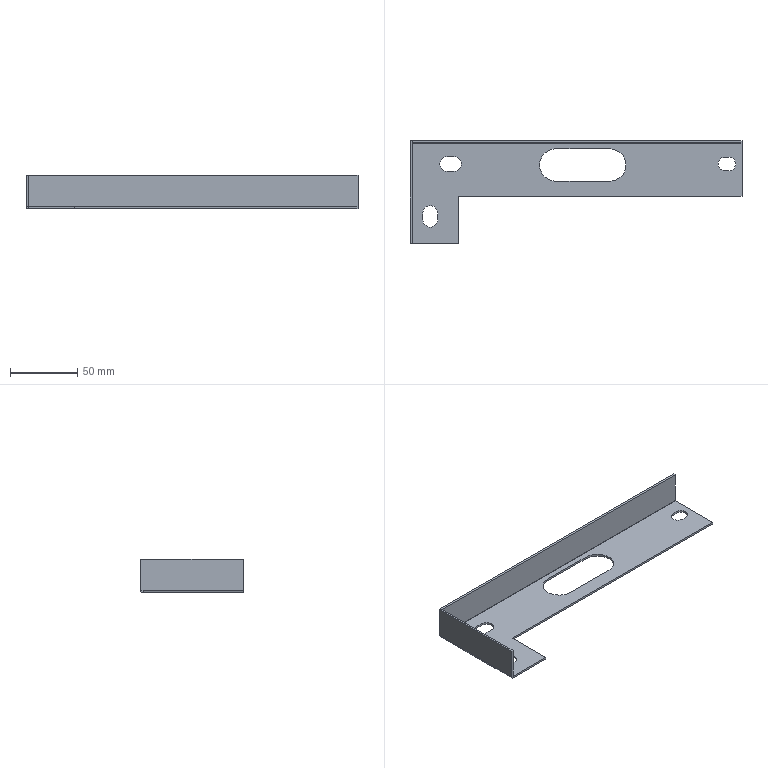Part | SolidWorks | features ICE 5, EdgeFlange 3, Cut 2, FlatPattern 1, SMBaseFlange 1, SheetMetal 1 | 1 solid | 44 faces | box 246 x 76 x 25 mm | volume 25378 mm3 | plane 29 | cylinder 15 | commonest cylinder face diameters 11 x5 10 x3 24 x3 0.4 x2 3.4 x2
STEP:
#1=CARTESIAN_POINT('',(37.,20.,-1.5));
#2=VERTEX_POINT('',#1);
#3=CARTESIAN_POINT('',(25.,32.,-1.5));
#4=VERTEX_POINT('',#3);
#5=CARTESIAN_POINT('',(25.,20.,-1.5));
#6=DIRECTION('',(0.,0.,1.));
#7=DIRECTION('',(1.,0.,0.));
#8=AXIS2_PLACEMENT_3D('',#5,#6,#7);
#9=CIRCLE('',#8,12.);
#10=EDGE_CURVE('',#2,#4,#9,.T.);
#11=ORIENTED_EDGE('',*,*,#10,.F.);
#12=CARTESIAN_POINT('',(37.,20.,0.));
#13=VERTEX_POINT('',#12);
#14=CARTESIAN_POINT('',(37.,20.,-10.));
#15=DIRECTION('',(0.,0.,1.));
#16=VECTOR('',#15,1000.);
#17=LINE('',#14,#16);
#18=EDGE_CURVE('',#2,#13,#17,.T.);
#19=ORIENTED_EDGE('',*,*,#18,.T.);
#20=CARTESIAN_POINT('',(25.,32.,0.));
#21=VERTEX_POINT('',#20);
#22=CARTESIAN_POINT('',(25.,20.,0.));
#23=DIRECTION('',(0.,0.,1.));
#24=DIRECTION('',(1.,0.,0.));
#25=AXIS2_PLACEMENT_3D('',#22,#23,#24);
#26=CIRCLE('',#25,12.);
#27=EDGE_CURVE('',#13,#21,#26,.T.);
#28=ORIENTED_EDGE('',*,*,#27,.T.);
#29=CARTESIAN_POINT('',(25.,32.,-10.));
#30=DIRECTION('',(0.,0.,1.));
#31=VECTOR('',#30,1000.);
#32=LINE('',#29,#31);
#33=EDGE_CURVE('',#4,#21,#32,.T.);
#34=ORIENTED_EDGE('',*,*,#33,.F.);
#35=EDGE_LOOP('',(#11,#19,#28,#34));
#36=FACE_OUTER_BOUND('',#35,.T.);
#37=CARTESIAN_POINT('',(25.,20.,-10.));
#38=DIRECTION('',(0.,0.,1.));
#39=DIRECTION('',(1.,0.,0.));
#40=AXIS2_PLACEMENT_3D('',#37,#38,#39);
#41=CYLINDRICAL_SURFACE('',#40,12.);
#42=ADVANCED_FACE('',(#36),#41,.F.);
#43=CARTESIAN_POINT('',(118.3,20.8,-1.5));
#44=VERTEX_POINT('',#43);
#45=CARTESIAN_POINT('',(113.3,25.8,-1.5));
#46=VERTEX_POINT('',#45);
#47=CARTESIAN_POINT('',(113.3,20.8,-1.5));
#48=DIRECTION('',(0.,0.,1.));
#49=DIRECTION('',(1.,0.,0.));
#50=AXIS2_PLACEMENT_3D('',#47,#48,#49);
#51=CIRCLE('',#50,5.);
#52=EDGE_CURVE('',#44,#46,#51,.T.);
#53=ORIENTED_EDGE('',*,*,#52,.F.);
#54=CARTESIAN_POINT('',(118.3,20.8,0.));
#55=VERTEX_POINT('',#54);
#56=CARTESIAN_POINT('',(118.3,20.8,-10.));
#57=DIRECTION('',(0.,0.,1.));
#58=VECTOR('',#57,1000.);
#59=LINE('',#56,#58);
#60=EDGE_CURVE('',#44,#55,#59,.T.);
#61=ORIENTED_EDGE('',*,*,#60,.T.);
#62=CARTESIAN_POINT('',(113.3,25.8,0.));
#63=VERTEX_POINT('',#62);
#64=CARTESIAN_POINT('',(113.3,20.8,0.));
#65=DIRECTION('',(0.,0.,1.));
#66=DIRECTION('',(1.,0.,0.));
#67=AXIS2_PLACEMENT_3D('',#64,#65,#66);
#68=CIRCLE('',#67,5.);
#69=EDGE_CURVE('',#55,#63,#68,.T.);
#70=ORIENTED_EDGE('',*,*,#69,.T.);
#71=CARTESIAN_POINT('',(113.3,25.8,-10.));
#72=DIRECTION('',(0.,0.,1.));
#73=VECTOR('',#72,1000.);
#74=LINE('',#71,#73);
#75=EDGE_CURVE('',#46,#63,#74,.T.);
#76=ORIENTED_EDGE('',*,*,#75,.F.);
#77=EDGE_LOOP('',(#53,#61,#70,#76));
#78=FACE_OUTER_BOUND('',#77,.T.);
#79=CARTESIAN_POINT('',(113.3,20.8,-10.));
#80=DIRECTION('',(0.,0.,1.));
#81=DIRECTION('',(1.,0.,0.));
#82=AXIS2_PLACEMENT_3D('',#79,#80,#81);
#83=CYLINDRICAL_SURFACE('',#82,5.);
#84=ADVANCED_FACE('',(#78),#83,.F.);
#85=CARTESIAN_POINT('',(-85.,20.8,-1.5));
#86=VERTEX_POINT('',#85);
#87=CARTESIAN_POINT('',(-90.5,26.3,-1.5));
#88=VERTEX_POINT('',#87);
#89=CARTESIAN_POINT('',(-90.5,20.8,-1.5));
#90=DIRECTION('',(0.,0.,1.));
#91=DIRECTION('',(1.,0.,0.));
#92=AXIS2_PLACEMENT_3D('',#89,#90,#91);
#93=CIRCLE('',#92,5.5);
#94=EDGE_CURVE('',#86,#88,#93,.T.);
#95=ORIENTED_EDGE('',*,*,#94,.F.);
#96=CARTESIAN_POINT('',(-85.,20.8,0.));
#97=VERTEX_POINT('',#96);
#98=CARTESIAN_POINT('',(-85.,20.8,-10.));
#99=DIRECTION('',(0.,0.,1.));
#100=VECTOR('',#99,1000.);
#101=LINE('',#98,#100);
#102=EDGE_CURVE('',#86,#97,#101,.T.);
#103=ORIENTED_EDGE('',*,*,#102,.T.);
#104=CARTESIAN_POINT('',(-90.5,26.3,0.));
#105=VERTEX_POINT('',#104);
#106=CARTESIAN_POINT('',(-90.5,20.8,0.));
#107=DIRECTION('',(0.,0.,1.));
#108=DIRECTION('',(1.,0.,0.));
#109=AXIS2_PLACEMENT_3D('',#106,#107,#108);
#110=CIRCLE('',#109,5.5);
#111=EDGE_CURVE('',#97,#105,#110,.T.);
#112=ORIENTED_EDGE('',*,*,#111,.T.);
#113=CARTESIAN_POINT('',(-90.5,26.3,-10.));
#114=DIRECTION('',(0.,0.,1.));
#115=VECTOR('',#114,1000.);
#116=LINE('',#113,#115);
#117=EDGE_CURVE('',#88,#105,#116,.T.);
#118=ORIENTED_EDGE('',*,*,#117,.F.);
#119=EDGE_LOOP('',(#95,#103,#112,#118));
#120=FACE_OUTER_BOUND('',#119,.T.);
#121=CARTESIAN_POINT('',(-90.5,20.8,-10.));
#122=DIRECTION('',(0.,0.,1.));
#123=DIRECTION('',(1.,0.,0.));
#124=AXIS2_PLACEMENT_3D('',#121,#122,#123);
#125=CYLINDRICAL_SURFACE('',#124,5.5);
#126=ADVANCED_FACE('',(#120),#125,.F.);
#127=CARTESIAN_POINT('',(-123.,36.3,0.2));
#128=VERTEX_POINT('',#127);
#129=CARTESIAN_POINT('',(-121.5,36.3,0.2));
#130=VERTEX_POINT('',#129);
#131=CARTESIAN_POINT('',(-123.,36.3,0.2));
#132=DIRECTION('',(1.,0.,0.));
#133=VECTOR('',#132,1000.);
#134=LINE('',#131,#133);
#135=EDGE_CURVE('',#128,#130,#134,.T.);
#136=ORIENTED_EDGE('',*,*,#135,.F.);
#137=CARTESIAN_POINT('',(-123.,38.,0.2));
#138=VERTEX_POINT('',#137);
#139=CARTESIAN_POINT('',(-123.,38.,0.2));
#140=DIRECTION('',(0.,1.,0.));
#141=VECTOR('',#140,1000.);
#142=LINE('',#139,#141);
#143=EDGE_CURVE('',#128,#138,#142,.T.);
#144=ORIENTED_EDGE('',*,*,#143,.T.);
#145=CARTESIAN_POINT('',(-121.5,38.,0.2));
#146=VERTEX_POINT('',#145);
#147=CARTESIAN_POINT('',(-123.,38.,0.2));
#148=DIRECTION('',(-1.,0.,0.));
#149=VECTOR('',#148,1000.);
#150=LINE('',#147,#149);
#151=EDGE_CURVE('',#146,#138,#150,.T.);
#152=ORIENTED_EDGE('',*,*,#151,.F.);
#153=CARTESIAN_POINT('',(-121.5,38.,0.2));
#154=DIRECTION('',(0.,-1.,0.));
#155=VECTOR('',#154,1000.);
#156=LINE('',#153,#155);
#157=EDGE_CURVE('',#146,#130,#156,.T.);
#158=ORIENTED_EDGE('',*,*,#157,.T.);
#159=EDGE_LOOP('',(#136,#144,#152,#158));
#160=FACE_OUTER_BOUND('',#159,.T.);
#161=CARTESIAN_POINT('',(0.,0.,0.2));
#162=DIRECTION('',(0.,0.,-1.));
#163=DIRECTION('',(-1.,0.,0.));
#164=AXIS2_PLACEMENT_3D('',#161,#162,#163);
#165=PLANE('',#164);
#166=ADVANCED_FACE('',(#160),#165,.T.);
#167=CARTESIAN_POINT('',(-123.,-38.,0.2));
#168=VERTEX_POINT('',#167);
#169=CARTESIAN_POINT('',(-123.,38.,0.2));
#170=DIRECTION('',(0.,1.,0.));
#171=VECTOR('',#170,1000.);
#172=LINE('',#169,#171);
#173=EDGE_CURVE('',#168,#128,#172,.T.);
#174=ORIENTED_EDGE('',*,*,#173,.T.);
#175=CARTESIAN_POINT('',(-121.3,36.3,-1.5));
#176=VERTEX_POINT('',#175);
#177=CARTESIAN_POINT('',(-121.3,36.3,0.2));
#178=DIRECTION('',(0.,-1.,0.));
#179=DIRECTION('',(0.,0.,1.));
#180=AXIS2_PLACEMENT_3D('',#177,#178,#179);
#181=CIRCLE('',#180,1.7);
#182=EDGE_CURVE('',#128,#176,#181,.T.);
#183=ORIENTED_EDGE('',*,*,#182,.T.);
#184=CARTESIAN_POINT('',(-121.3,-38.,-1.5));
#185=VERTEX_POINT('',#184);
#186=CARTESIAN_POINT('',(-121.3,-38.,-1.5));
#187=DIRECTION('',(0.,1.,0.));
#188=VECTOR('',#187,1000.);
#189=LINE('',#186,#188);
#190=EDGE_CURVE('',#185,#176,#189,.T.);
#191=ORIENTED_EDGE('',*,*,#190,.F.);
#192=CARTESIAN_POINT('',(-121.3,-38.,0.2));
#193=DIRECTION('',(0.,-1.,0.));
#194=DIRECTION('',(0.,0.,-1.));
#195=AXIS2_PLACEMENT_3D('',#192,#193,#194);
#196=CIRCLE('',#195,1.7);
#197=EDGE_CURVE('',#168,#185,#196,.T.);
#198=ORIENTED_EDGE('',*,*,#197,.F.);
#199=EDGE_LOOP('',(#174,#183,#191,#198));
#200=FACE_OUTER_BOUND('',#199,.T.);
#201=CARTESIAN_POINT('',(-121.3,-38.,0.2));
#202=DIRECTION('',(0.,-1.,0.));
#203=DIRECTION('',(-1.,0.,0.));
#204=AXIS2_PLACEMENT_3D('',#201,#202,#203);
#205=CYLINDRICAL_SURFACE('',#204,1.7);
#206=ADVANCED_FACE('',(#200),#205,.T.);
#207=CARTESIAN_POINT('',(-15.,32.,-1.5));
#208=VERTEX_POINT('',#207);
#209=CARTESIAN_POINT('',(0.,32.,-1.5));
#210=DIRECTION('',(-1.,0.,0.));
#211=VECTOR('',#210,1000.);
#212=LINE('',#209,#211);
#213=EDGE_CURVE('',#4,#208,#212,.T.);
#214=ORIENTED_EDGE('',*,*,#213,.T.);
#215=CARTESIAN_POINT('',(-15.,8.,-1.5));
#216=VERTEX_POINT('',#215);
#217=CARTESIAN_POINT('',(-15.,20.,-1.5));
#218=DIRECTION('',(0.,0.,1.));
#219=DIRECTION('',(1.,0.,0.));
#220=AXIS2_PLACEMENT_3D('',#217,#218,#219);
#221=CIRCLE('',#220,12.);
#222=EDGE_CURVE('',#208,#216,#221,.T.);
#223=ORIENTED_EDGE('',*,*,#222,.T.);
#224=CARTESIAN_POINT('',(25.,8.,-1.5));
#225=VERTEX_POINT('',#224);
#226=CARTESIAN_POINT('',(0.,8.,-1.5));
#227=DIRECTION('',(1.,0.,0.));
#228=VECTOR('',#227,1000.);
#229=LINE('',#226,#228);
#230=EDGE_CURVE('',#216,#225,#229,.T.);
#231=ORIENTED_EDGE('',*,*,#230,.T.);
#232=CARTESIAN_POINT('',(25.,20.,-1.5));
#233=DIRECTION('',(0.,0.,1.));
#234=DIRECTION('',(1.,0.,0.));
#235=AXIS2_PLACEMENT_3D('',#232,#233,#234);
#236=CIRCLE('',#235,12.);
#237=EDGE_CURVE('',#225,#2,#236,.T.);
#238=ORIENTED_EDGE('',*,*,#237,.T.);
#239=ORIENTED_EDGE('',*,*,#10,.T.);
#240=EDGE_LOOP('',(#214,#223,#231,#238,#239));
#241=FACE_BOUND('',#240,.T.);
#242=CARTESIAN_POINT('',(110.3,25.8,-1.5));
#243=VERTEX_POINT('',#242);
#244=CARTESIAN_POINT('',(0.,25.8,-1.5));
#245=DIRECTION('',(-1.,0.,0.));
#246=VECTOR('',#245,1000.);
#247=LINE('',#244,#246);
#248=EDGE_CURVE('',#46,#243,#247,.T.);
#249=ORIENTED_EDGE('',*,*,#248,.T.);
#250=CARTESIAN_POINT('',(110.3,15.8,-1.5));
#251=VERTEX_POINT('',#250);
#252=CARTESIAN_POINT('',(110.3,20.8,-1.5));
#253=DIRECTION('',(0.,0.,1.));
#254=DIRECTION('',(1.,0.,0.));
#255=AXIS2_PLACEMENT_3D('',#252,#253,#254);
#256=CIRCLE('',#255,5.);
#257=EDGE_CURVE('',#243,#251,#256,.T.);
#258=ORIENTED_EDGE('',*,*,#257,.T.);
#259=CARTESIAN_POINT('',(113.3,15.8,-1.5));
#260=VERTEX_POINT('',#259);
#261=CARTESIAN_POINT('',(0.,15.8,-1.5));
#262=DIRECTION('',(1.,0.,0.));
#263=VECTOR('',#262,1000.);
#264=LINE('',#261,#263);
#265=EDGE_CURVE('',#251,#260,#264,.T.);
#266=ORIENTED_EDGE('',*,*,#265,.T.);
#267=CARTESIAN_POINT('',(113.3,20.8,-1.5));
#268=DIRECTION('',(0.,0.,1.));
#269=DIRECTION('',(1.,0.,0.));
#270=AXIS2_PLACEMENT_3D('',#267,#268,#269);
#271=CIRCLE('',#270,5.);
#272=EDGE_CURVE('',#260,#44,#271,.T.);
#273=ORIENTED_EDGE('',*,*,#272,.T.);
#274=ORIENTED_EDGE('',*,*,#52,.T.);
#275=EDGE_LOOP('',(#249,#258,#266,#273,#274));
#276=FACE_BOUND('',#275,.T.);
#277=CARTESIAN_POINT('',(-95.5,26.3,-1.5));
#278=VERTEX_POINT('',#277);
#279=CARTESIAN_POINT('',(0.,26.3,-1.5));
#280=DIRECTION('',(-1.,0.,0.));
#281=VECTOR('',#280,1000.);
#282=LINE('',#279,#281);
#283=EDGE_CURVE('',#88,#278,#282,.T.);
#284=ORIENTED_EDGE('',*,*,#283,.T.);
#285=CARTESIAN_POINT('',(-95.5,15.3,-1.5));
#286=VERTEX_POINT('',#285);
#287=CARTESIAN_POINT('',(-95.5,20.8,-1.5));
#288=DIRECTION('',(0.,0.,1.));
#289=DIRECTION('',(1.,0.,0.));
#290=AXIS2_PLACEMENT_3D('',#287,#288,#289);
#291=CIRCLE('',#290,5.5);
#292=EDGE_CURVE('',#278,#286,#291,.T.);
#293=ORIENTED_EDGE('',*,*,#292,.T.);
#294=CARTESIAN_POINT('',(-90.5,15.3,-1.5));
#295=VERTEX_POINT('',#294);
#296=CARTESIAN_POINT('',(0.,15.3,-1.5));
#297=DIRECTION('',(1.,0.,0.));
#298=VECTOR('',#297,1000.);
#299=LINE('',#296,#298);
#300=EDGE_CURVE('',#286,#295,#299,.T.);
#301=ORIENTED_EDGE('',*,*,#300,.T.);
#302=CARTESIAN_POINT('',(-90.5,20.8,-1.5));
#303=DIRECTION('',(0.,0.,1.));
#304=DIRECTION('',(1.,0.,0.));
#305=AXIS2_PLACEMENT_3D('',#302,#303,#304);
#306=CIRCLE('',#305,5.5);
#307=EDGE_CURVE('',#295,#86,#306,.T.);
#308=ORIENTED_EDGE('',*,*,#307,.T.);
#309=ORIENTED_EDGE('',*,*,#94,.T.);
#310=EDGE_LOOP('',(#284,#293,#301,#308,#309));
#311=FACE_BOUND('',#310,.T.);
#312=CARTESIAN_POINT('',(-102.5,-20.5,-1.5));
#313=VERTEX_POINT('',#312);
#314=CARTESIAN_POINT('',(-102.5,-15.5,-1.5));
#315=VERTEX_POINT('',#314);
#316=CARTESIAN_POINT('',(-102.5,0.,-1.5));
#317=DIRECTION('',(0.,1.,0.));
#318=VECTOR('',#317,1000.);
#319=LINE('',#316,#318);
#320=EDGE_CURVE('',#313,#315,#319,.T.);
#321=ORIENTED_EDGE('',*,*,#320,.T.);
#322=CARTESIAN_POINT('',(-113.5,-15.5,-1.5));
#323=VERTEX_POINT('',#322);
#324=CARTESIAN_POINT('',(-108.,-15.5,-1.5));
#325=DIRECTION('',(0.,0.,1.));
#326=DIRECTION('',(1.,0.,0.));
#327=AXIS2_PLACEMENT_3D('',#324,#325,#326);
#328=CIRCLE('',#327,5.5);
#329=EDGE_CURVE('',#315,#323,#328,.T.);
#330=ORIENTED_EDGE('',*,*,#329,.T.);
#331=CARTESIAN_POINT('',(-113.5,-20.5,-1.5));
#332=VERTEX_POINT('',#331);
#333=CARTESIAN_POINT('',(-113.5,0.,-1.5));
#334=DIRECTION('',(0.,-1.,0.));
#335=VECTOR('',#334,1000.);
#336=LINE('',#333,#335);
#337=EDGE_CURVE('',#323,#332,#336,.T.);
#338=ORIENTED_EDGE('',*,*,#337,.T.);
#339=CARTESIAN_POINT('',(-108.,-20.5,-1.5));
#340=DIRECTION('',(0.,0.,1.));
#341=DIRECTION('',(1.,0.,0.));
#342=AXIS2_PLACEMENT_3D('',#339,#340,#341);
#343=CIRCLE('',#342,5.5);
#344=EDGE_CURVE('',#332,#313,#343,.T.);
#345=ORIENTED_EDGE('',*,*,#344,.T.);
#346=EDGE_LOOP('',(#321,#330,#338,#345));
#347=FACE_BOUND('',#346,.T.);
#348=CARTESIAN_POINT('',(123.,-3.,-1.5));
#349=VERTEX_POINT('',#348);
#350=CARTESIAN_POINT('',(123.,36.3,-1.5));
#351=VERTEX_POINT('',#350);
#352=CARTESIAN_POINT('',(123.,38.,-1.5));
#353=DIRECTION('',(0.,1.,0.));
#354=VECTOR('',#353,1000.);
#355=LINE('',#352,#354);
#356=EDGE_CURVE('',#349,#351,#355,.T.);
#357=ORIENTED_EDGE('',*,*,#356,.F.);
#358=CARTESIAN_POINT('',(-87.,-3.,-1.5));
#359=VERTEX_POINT('',#358);
#360=CARTESIAN_POINT('',(123.,-3.,-1.5));
#361=DIRECTION('',(1.,0.,0.));
#362=VECTOR('',#361,1000.);
#363=LINE('',#360,#362);
#364=EDGE_CURVE('',#359,#349,#363,.T.);
#365=ORIENTED_EDGE('',*,*,#364,.F.);
#366=CARTESIAN_POINT('',(-87.,-38.,-1.5));
#367=VERTEX_POINT('',#366);
#368=CARTESIAN_POINT('',(-87.,-38.,-1.5));
#369=DIRECTION('',(0.,1.,0.));
#370=VECTOR('',#369,1000.);
#371=LINE('',#368,#370);
#372=EDGE_CURVE('',#367,#359,#371,.T.);
#373=ORIENTED_EDGE('',*,*,#372,.F.);
#374=CARTESIAN_POINT('',(-123.,-38.,-1.5));
#375=DIRECTION('',(1.,0.,0.));
#376=VECTOR('',#375,1000.);
#377=LINE('',#374,#376);
#378=EDGE_CURVE('',#185,#367,#377,.T.);
#379=ORIENTED_EDGE('',*,*,#378,.F.);
#380=ORIENTED_EDGE('',*,*,#190,.T.);
#381=CARTESIAN_POINT('',(-121.3,36.3,-1.5));
#382=DIRECTION('',(1.,0.,0.));
#383=VECTOR('',#382,1000.);
#384=LINE('',#381,#383);
#385=EDGE_CURVE('',#176,#351,#384,.T.);
#386=ORIENTED_EDGE('',*,*,#385,.T.);
#387=EDGE_LOOP('',(#357,#365,#373,#379,#380,#386));
#388=FACE_OUTER_BOUND('',#387,.T.);
#389=CARTESIAN_POINT('',(0.,0.,-1.5));
#390=DIRECTION('',(0.,0.,1.));
#391=DIRECTION('',(1.,0.,0.));
#392=AXIS2_PLACEMENT_3D('',#389,#390,#391);
#393=PLANE('',#392);
#394=ADVANCED_FACE('',(#241,#276,#311,#347,#388),#393,.F.);
#395=CARTESIAN_POINT('',(123.,-3.,0.));
#396=VERTEX_POINT('',#395);
#397=CARTESIAN_POINT('',(-87.,-3.,0.));
#398=VERTEX_POINT('',#397);
#399=CARTESIAN_POINT('',(0.,-3.,0.));
#400=DIRECTION('',(-1.,0.,0.));
#401=VECTOR('',#400,1000.);
#402=LINE('',#399,#401);
#403=EDGE_CURVE('',#396,#398,#402,.T.);
#404=ORIENTED_EDGE('',*,*,#403,.F.);
#405=CARTESIAN_POINT('',(123.,36.3,0.));
#406=VERTEX_POINT('',#405);
#407=CARTESIAN_POINT('',(123.,38.,0.));
#408=DIRECTION('',(0.,1.,0.));
#409=VECTOR('',#408,1000.);
#410=LINE('',#407,#409);
#411=EDGE_CURVE('',#396,#406,#410,.T.);
#412=ORIENTED_EDGE('',*,*,#411,.T.);
#413=CARTESIAN_POINT('',(-121.3,36.3,0.));
#414=VERTEX_POINT('',#413);
#415=CARTESIAN_POINT('',(-121.3,36.3,0.));
#416=DIRECTION('',(1.,0.,0.));
#417=VECTOR('',#416,1000.);
#418=LINE('',#415,#417);
#419=EDGE_CURVE('',#414,#406,#418,.T.);
#420=ORIENTED_EDGE('',*,*,#419,.F.);
#421=CARTESIAN_POINT('',(-121.3,-38.,0.));
#422=VERTEX_POINT('',#421);
#423=CARTESIAN_POINT('',(-121.3,-38.,0.));
#424=DIRECTION('',(0.,1.,0.));
#425=VECTOR('',#424,1000.);
#426=LINE('',#423,#425);
#427=EDGE_CURVE('',#422,#414,#426,.T.);
#428=ORIENTED_EDGE('',*,*,#427,.F.);
#429=CARTESIAN_POINT('',(-87.,-38.,0.));
#430=VERTEX_POINT('',#429);
#431=CARTESIAN_POINT('',(-123.,-38.,0.));
#432=DIRECTION('',(1.,0.,0.));
#433=VECTOR('',#432,1000.);
#434=LINE('',#431,#433);
#435=EDGE_CURVE('',#422,#430,#434,.T.);
#436=ORIENTED_EDGE('',*,*,#435,.T.);
#437=CARTESIAN_POINT('',(-87.,0.,0.));
#438=DIRECTION('',(0.,-1.,0.));
#439=VECTOR('',#438,1000.);
#440=LINE('',#437,#439);
#441=EDGE_CURVE('',#398,#430,#440,.T.);
#442=ORIENTED_EDGE('',*,*,#441,.F.);
#443=EDGE_LOOP('',(#404,#412,#420,#428,#436,#442));
#444=FACE_OUTER_BOUND('',#443,.T.);
#445=CARTESIAN_POINT('',(-15.,32.,0.));
#446=VERTEX_POINT('',#445);
#447=CARTESIAN_POINT('',(-15.,8.,0.));
#448=VERTEX_POINT('',#447);
#449=CARTESIAN_POINT('',(-15.,20.,0.));
#450=DIRECTION('',(0.,0.,1.));
#451=DIRECTION('',(1.,0.,0.));
#452=AXIS2_PLACEMENT_3D('',#449,#450,#451);
#453=CIRCLE('',#452,12.);
#454=EDGE_CURVE('',#446,#448,#453,.T.);
#455=ORIENTED_EDGE('',*,*,#454,.F.);
#456=CARTESIAN_POINT('',(-15.,32.,0.));
#457=DIRECTION('',(-1.,0.,0.));
#458=VECTOR('',#457,1000.);
#459=LINE('',#456,#458);
#460=EDGE_CURVE('',#21,#446,#459,.T.);
#461=ORIENTED_EDGE('',*,*,#460,.F.);
#462=ORIENTED_EDGE('',*,*,#27,.F.);
#463=CARTESIAN_POINT('',(25.,8.,0.));
#464=VERTEX_POINT('',#463);
#465=CARTESIAN_POINT('',(25.,20.,0.));
#466=DIRECTION('',(0.,0.,1.));
#467=DIRECTION('',(1.,0.,0.));
#468=AXIS2_PLACEMENT_3D('',#465,#466,#467);
#469=CIRCLE('',#468,12.);
#470=EDGE_CURVE('',#464,#13,#469,.T.);
#471=ORIENTED_EDGE('',*,*,#470,.F.);
#472=CARTESIAN_POINT('',(-15.,8.,0.));
#473=DIRECTION('',(1.,0.,0.));
#474=VECTOR('',#473,1000.);
#475=LINE('',#472,#474);
#476=EDGE_CURVE('',#448,#464,#475,.T.);
#477=ORIENTED_EDGE('',*,*,#476,.F.);
#478=EDGE_LOOP('',(#455,#461,#462,#471,#477));
#479=FACE_BOUND('',#478,.T.);
#480=CARTESIAN_POINT('',(110.3,25.8,0.));
#481=VERTEX_POINT('',#480);
#482=CARTESIAN_POINT('',(110.3,15.8,0.));
#483=VERTEX_POINT('',#482);
#484=CARTESIAN_POINT('',(110.3,20.8,0.));
#485=DIRECTION('',(0.,0.,1.));
#486=DIRECTION('',(1.,0.,0.));
#487=AXIS2_PLACEMENT_3D('',#484,#485,#486);
#488=CIRCLE('',#487,5.);
#489=EDGE_CURVE('',#481,#483,#488,.T.);
#490=ORIENTED_EDGE('',*,*,#489,.F.);
#491=CARTESIAN_POINT('',(110.3,25.8,0.));
#492=DIRECTION('',(-1.,0.,0.));
#493=VECTOR('',#492,1000.);
#494=LINE('',#491,#493);
#495=EDGE_CURVE('',#63,#481,#494,.T.);
#496=ORIENTED_EDGE('',*,*,#495,.F.);
#497=ORIENTED_EDGE('',*,*,#69,.F.);
#498=CARTESIAN_POINT('',(113.3,15.8,0.));
#499=VERTEX_POINT('',#498);
#500=CARTESIAN_POINT('',(113.3,20.8,0.));
#501=DIRECTION('',(0.,0.,1.));
#502=DIRECTION('',(1.,0.,0.));
#503=AXIS2_PLACEMENT_3D('',#500,#501,#502);
#504=CIRCLE('',#503,5.);
#505=EDGE_CURVE('',#499,#55,#504,.T.);
#506=ORIENTED_EDGE('',*,*,#505,.F.);
#507=CARTESIAN_POINT('',(110.3,15.8,0.));
#508=DIRECTION('',(1.,0.,0.));
#509=VECTOR('',#508,1000.);
#510=LINE('',#507,#509);
#511=EDGE_CURVE('',#483,#499,#510,.T.);
#512=ORIENTED_EDGE('',*,*,#511,.F.);
#513=EDGE_LOOP('',(#490,#496,#497,#506,#512));
#514=FACE_BOUND('',#513,.T.);
#515=CARTESIAN_POINT('',(-95.5,26.3,0.));
#516=VERTEX_POINT('',#515);
#517=CARTESIAN_POINT('',(-95.5,15.3,0.));
#518=VERTEX_POINT('',#517);
#519=CARTESIAN_POINT('',(-95.5,20.8,0.));
#520=DIRECTION('',(0.,0.,1.));
#521=DIRECTION('',(1.,0.,0.));
#522=AXIS2_PLACEMENT_3D('',#519,#520,#521);
#523=CIRCLE('',#522,5.5);
#524=EDGE_CURVE('',#516,#518,#523,.T.);
#525=ORIENTED_EDGE('',*,*,#524,.F.);
#526=CARTESIAN_POINT('',(-95.5,26.3,0.));
#527=DIRECTION('',(-1.,0.,0.));
#528=VECTOR('',#527,1000.);
#529=LINE('',#526,#528);
#530=EDGE_CURVE('',#105,#516,#529,.T.);
#531=ORIENTED_EDGE('',*,*,#530,.F.);
#532=ORIENTED_EDGE('',*,*,#111,.F.);
#533=CARTESIAN_POINT('',(-90.5,15.3,0.));
#534=VERTEX_POINT('',#533);
#535=CARTESIAN_POINT('',(-90.5,20.8,0.));
#536=DIRECTION('',(0.,0.,1.));
#537=DIRECTION('',(1.,0.,0.));
#538=AXIS2_PLACEMENT_3D('',#535,#536,#537);
#539=CIRCLE('',#538,5.5);
#540=EDGE_CURVE('',#534,#97,#539,.T.);
#541=ORIENTED_EDGE('',*,*,#540,.F.);
#542=CARTESIAN_POINT('',(-95.5,15.3,0.));
#543=DIRECTION('',(1.,0.,0.));
#544=VECTOR('',#543,1000.);
#545=LINE('',#542,#544);
#546=EDGE_CURVE('',#518,#534,#545,.T.);
#547=ORIENTED_EDGE('',*,*,#546,.F.);
#548=EDGE_LOOP('',(#525,#531,#532,#541,#547));
#549=FACE_BOUND('',#548,.T.);
#550=CARTESIAN_POINT('',(-102.5,-15.5,0.));
#551=VERTEX_POINT('',#550);
#552=CARTESIAN_POINT('',(-113.5,-15.5,0.));
#553=VERTEX_POINT('',#552);
#554=CARTESIAN_POINT('',(-108.,-15.5,0.));
#555=DIRECTION('',(0.,0.,1.));
#556=DIRECTION('',(1.,0.,0.));
#557=AXIS2_PLACEMENT_3D('',#554,#555,#556);
#558=CIRCLE('',#557,5.5);
#559=EDGE_CURVE('',#551,#553,#558,.T.);
#560=ORIENTED_EDGE('',*,*,#559,.F.);
#561=CARTESIAN_POINT('',(-102.5,-20.5,0.));
#562=VERTEX_POINT('',#561);
#563=CARTESIAN_POINT('',(-102.5,-15.5,0.));
#564=DIRECTION('',(0.,1.,0.));
#565=VECTOR('',#564,1000.);
#566=LINE('',#563,#565);
#567=EDGE_CURVE('',#562,#551,#566,.T.);
#568=ORIENTED_EDGE('',*,*,#567,.F.);
#569=CARTESIAN_POINT('',(-113.5,-20.5,0.));
#570=VERTEX_POINT('',#569);
#571=CARTESIAN_POINT('',(-108.,-20.5,0.));
#572=DIRECTION('',(0.,0.,1.));
#573=DIRECTION('',(1.,0.,0.));
#574=AXIS2_PLACEMENT_3D('',#571,#572,#573);
#575=CIRCLE('',#574,5.5);
#576=EDGE_CURVE('',#570,#562,#575,.T.);
#577=ORIENTED_EDGE('',*,*,#576,.F.);
#578=CARTESIAN_POINT('',(-113.5,-15.5,0.));
#579=DIRECTION('',(0.,-1.,0.));
#580=VECTOR('',#579,1000.);
#581=LINE('',#578,#580);
#582=EDGE_CURVE('',#553,#570,#581,.T.);
#583=ORIENTED_EDGE('',*,*,#582,.F.);
#584=EDGE_LOOP('',(#560,#568,#577,#583));
#585=FACE_BOUND('',#584,.T.);
#586=CARTESIAN_POINT('',(0.,0.,0.));
#587=DIRECTION('',(0.,0.,1.));
#588=DIRECTION('',(1.,0.,0.));
#589=AXIS2_PLACEMENT_3D('',#586,#587,#588);
#590=PLANE('',#589);
#591=ADVANCED_FACE('',(#444,#479,#514,#549,#585),#590,.T.);
#592=CARTESIAN_POINT('',(-87.,-38.,8.5));
#593=DIRECTION('',(0.,0.,-1.));
#594=VECTOR('',#593,1000.);
#595=LINE('',#592,#594);
#596=EDGE_CURVE('',#430,#367,#595,.T.);
#597=ORIENTED_EDGE('',*,*,#596,.F.);
#598=ORIENTED_EDGE('',*,*,#435,.F.);
#599=CARTESIAN_POINT('',(-121.3,-38.,0.));
#600=DIRECTION('',(0.,0.,-1.));
#601=VECTOR('',#600,1000.);
#602=LINE('',#599,#601);
#603=EDGE_CURVE('',#422,#185,#602,.T.);
#604=ORIENTED_EDGE('',*,*,#603,.T.);
#605=ORIENTED_EDGE('',*,*,#378,.T.);
#606=EDGE_LOOP('',(#597,#598,#604,#605));
#607=FACE_OUTER_BOUND('',#606,.T.);
#608=CARTESIAN_POINT('',(-123.,-38.,-1.5));
#609=DIRECTION('',(0.,-1.,0.));
#610=DIRECTION('',(0.,0.,-1.));
#611=AXIS2_PLACEMENT_3D('',#608,#609,#610);
#612=PLANE('',#611);
#613=ADVANCED_FACE('',(#607),#612,.T.);
#614=CARTESIAN_POINT('',(123.,-3.,-1.5));
#615=DIRECTION('',(0.,0.,1.));
#616=VECTOR('',#615,1000.);
#617=LINE('',#614,#616);
#618=EDGE_CURVE('',#349,#396,#617,.T.);
#619=ORIENTED_EDGE('',*,*,#618,.F.);
#620=ORIENTED_EDGE('',*,*,#356,.T.);
#621=CARTESIAN_POINT('',(123.,36.3,0.));
#622=DIRECTION('',(0.,0.,-1.));
#623=VECTOR('',#622,1000.);
#624=LINE('',#621,#623);
#625=EDGE_CURVE('',#406,#351,#624,.T.);
#626=ORIENTED_EDGE('',*,*,#625,.F.);
#627=ORIENTED_EDGE('',*,*,#411,.F.);
#628=EDGE_LOOP('',(#619,#620,#626,#627));
#629=FACE_OUTER_BOUND('',#628,.T.);
#630=CARTESIAN_POINT('',(123.,38.,-1.5));
#631=DIRECTION('',(1.,0.,0.));
#632=DIRECTION('',(0.,0.,-1.));
#633=AXIS2_PLACEMENT_3D('',#630,#631,#632);
#634=PLANE('',#633);
#635=ADVANCED_FACE('',(#629),#634,.T.);
#636=CARTESIAN_POINT('',(-102.5,-15.5,-10.));
#637=DIRECTION('',(0.,0.,1.));
#638=VECTOR('',#637,1000.);
#639=LINE('',#636,#638);
#640=EDGE_CURVE('',#315,#551,#639,.T.);
#641=ORIENTED_EDGE('',*,*,#640,.T.);
#642=ORIENTED_EDGE('',*,*,#559,.T.);
#643=CARTESIAN_POINT('',(-113.5,-15.5,-10.));
#644=DIRECTION('',(0.,0.,1.));
#645=VECTOR('',#644,1000.);
#646=LINE('',#643,#645);
#647=EDGE_CURVE('',#323,#553,#646,.T.);
#648=ORIENTED_EDGE('',*,*,#647,.F.);
#649=ORIENTED_EDGE('',*,*,#329,.F.);
#650=EDGE_LOOP('',(#641,#642,#648,#649));
#651=FACE_OUTER_BOUND('',#650,.T.);
#652=CARTESIAN_POINT('',(-108.,-15.5,-10.));
#653=DIRECTION('',(0.,0.,1.));
#654=DIRECTION('',(1.,0.,0.));
#655=AXIS2_PLACEMENT_3D('',#652,#653,#654);
#656=CYLINDRICAL_SURFACE('',#655,5.5);
#657=ADVANCED_FACE('',(#651),#656,.F.);
#658=CARTESIAN_POINT('',(-102.5,-20.5,-10.));
#659=DIRECTION('',(0.,0.,1.));
#660=VECTOR('',#659,1000.);
#661=LINE('',#658,#660);
#662=EDGE_CURVE('',#313,#562,#661,.T.);
#663=ORIENTED_EDGE('',*,*,#662,.T.);
#664=ORIENTED_EDGE('',*,*,#567,.T.);
#665=ORIENTED_EDGE('',*,*,#640,.F.);
#666=ORIENTED_EDGE('',*,*,#320,.F.);
#667=EDGE_LOOP('',(#663,#664,#665,#666));
#668=FACE_OUTER_BOUND('',#667,.T.);
#669=CARTESIAN_POINT('',(-102.5,-15.5,-10.));
#670=DIRECTION('',(1.,0.,0.));
#671=DIRECTION('',(0.,0.,-1.));
#672=AXIS2_PLACEMENT_3D('',#669,#670,#671);
#673=PLANE('',#672);
#674=ADVANCED_FACE('',(#668),#673,.F.);
#675=CARTESIAN_POINT('',(-113.5,-20.5,-10.));
#676=DIRECTION('',(0.,0.,1.));
#677=VECTOR('',#676,1000.);
#678=LINE('',#675,#677);
#679=EDGE_CURVE('',#332,#570,#678,.T.);
#680=ORIENTED_EDGE('',*,*,#679,.T.);
#681=ORIENTED_EDGE('',*,*,#576,.T.);
#682=ORIENTED_EDGE('',*,*,#662,.F.);
#683=ORIENTED_EDGE('',*,*,#344,.F.);
#684=EDGE_LOOP('',(#680,#681,#682,#683));
#685=FACE_OUTER_BOUND('',#684,.T.);
#686=CARTESIAN_POINT('',(-108.,-20.5,-10.));
#687=DIRECTION('',(0.,0.,1.));
#688=DIRECTION('',(1.,0.,0.));
#689=AXIS2_PLACEMENT_3D('',#686,#687,#688);
#690=CYLINDRICAL_SURFACE('',#689,5.5);
#691=ADVANCED_FACE('',(#685),#690,.F.);
#692=ORIENTED_EDGE('',*,*,#647,.T.);
#693=ORIENTED_EDGE('',*,*,#582,.T.);
#694=ORIENTED_EDGE('',*,*,#679,.F.);
#695=ORIENTED_EDGE('',*,*,#337,.F.);
#696=EDGE_LOOP('',(#692,#693,#694,#695));
#697=FACE_OUTER_BOUND('',#696,.T.);
#698=CARTESIAN_POINT('',(-113.5,-15.5,-10.));
#699=DIRECTION('',(-1.,0.,0.));
#700=DIRECTION('',(0.,0.,1.));
#701=AXIS2_PLACEMENT_3D('',#698,#699,#700);
#702=PLANE('',#701);
#703=ADVANCED_FACE('',(#697),#702,.F.);
#704=CARTESIAN_POINT('',(-95.5,26.3,-10.));
#705=DIRECTION('',(0.,0.,1.));
#706=VECTOR('',#705,1000.);
#707=LINE('',#704,#706);
#708=EDGE_CURVE('',#278,#516,#707,.T.);
#709=ORIENTED_EDGE('',*,*,#708,.T.);
#710=ORIENTED_EDGE('',*,*,#524,.T.);
#711=CARTESIAN_POINT('',(-95.5,15.3,-10.));
#712=DIRECTION('',(0.,0.,1.));
#713=VECTOR('',#712,1000.);
#714=LINE('',#711,#713);
#715=EDGE_CURVE('',#286,#518,#714,.T.);
#716=ORIENTED_EDGE('',*,*,#715,.F.);
#717=ORIENTED_EDGE('',*,*,#292,.F.);
#718=EDGE_LOOP('',(#709,#710,#716,#717));
#719=FACE_OUTER_BOUND('',#718,.T.);
#720=CARTESIAN_POINT('',(-95.5,20.8,-10.));
#721=DIRECTION('',(0.,0.,1.));
#722=DIRECTION('',(1.,0.,0.));
#723=AXIS2_PLACEMENT_3D('',#720,#721,#722);
#724=CYLINDRICAL_SURFACE('',#723,5.5);
#725=ADVANCED_FACE('',(#719),#724,.F.);
#726=ORIENTED_EDGE('',*,*,#117,.T.);
#727=ORIENTED_EDGE('',*,*,#530,.T.);
#728=ORIENTED_EDGE('',*,*,#708,.F.);
#729=ORIENTED_EDGE('',*,*,#283,.F.);
#730=EDGE_LOOP('',(#726,#727,#728,#729));
#731=FACE_OUTER_BOUND('',#730,.T.);
#732=CARTESIAN_POINT('',(-95.5,26.3,-10.));
#733=DIRECTION('',(0.,1.,0.));
#734=DIRECTION('',(0.,0.,1.));
#735=AXIS2_PLACEMENT_3D('',#732,#733,#734);
#736=PLANE('',#735);
#737=ADVANCED_FACE('',(#731),#736,.F.);
#738=ORIENTED_EDGE('',*,*,#102,.F.);
#739=ORIENTED_EDGE('',*,*,#307,.F.);
#740=CARTESIAN_POINT('',(-90.5,15.3,-10.));
#741=DIRECTION('',(0.,0.,1.));
#742=VECTOR('',#741,1000.);
#743=LINE('',#740,#742);
#744=EDGE_CURVE('',#295,#534,#743,.T.);
#745=ORIENTED_EDGE('',*,*,#744,.T.);
#746=ORIENTED_EDGE('',*,*,#540,.T.);
#747=EDGE_LOOP('',(#738,#739,#745,#746));
#748=FACE_OUTER_BOUND('',#747,.T.);
#749=CARTESIAN_POINT('',(-90.5,20.8,-10.));
#750=DIRECTION('',(0.,0.,1.));
#751=DIRECTION('',(1.,0.,0.));
#752=AXIS2_PLACEMENT_3D('',#749,#750,#751);
#753=CYLINDRICAL_SURFACE('',#752,5.5);
#754=ADVANCED_FACE('',(#748),#753,.F.);
#755=ORIENTED_EDGE('',*,*,#715,.T.);
#756=ORIENTED_EDGE('',*,*,#546,.T.);
#757=ORIENTED_EDGE('',*,*,#744,.F.);
#758=ORIENTED_EDGE('',*,*,#300,.F.);
#759=EDGE_LOOP('',(#755,#756,#757,#758));
#760=FACE_OUTER_BOUND('',#759,.T.);
#761=CARTESIAN_POINT('',(-95.5,15.3,-10.));
#762=DIRECTION('',(0.,-1.,0.));
#763=DIRECTION('',(1.,0.,0.));
#764=AXIS2_PLACEMENT_3D('',#761,#762,#763);
#765=PLANE('',#764);
#766=ADVANCED_FACE('',(#760),#765,.F.);
#767=CARTESIAN_POINT('',(110.3,25.8,-10.));
#768=DIRECTION('',(0.,0.,1.));
#769=VECTOR('',#768,1000.);
#770=LINE('',#767,#769);
#771=EDGE_CURVE('',#243,#481,#770,.T.);
#772=ORIENTED_EDGE('',*,*,#771,.T.);
#773=ORIENTED_EDGE('',*,*,#489,.T.);
#774=CARTESIAN_POINT('',(110.3,15.8,-10.));
#775=DIRECTION('',(0.,0.,1.));
#776=VECTOR('',#775,1000.);
#777=LINE('',#774,#776);
#778=EDGE_CURVE('',#251,#483,#777,.T.);
#779=ORIENTED_EDGE('',*,*,#778,.F.);
#780=ORIENTED_EDGE('',*,*,#257,.F.);
#781=EDGE_LOOP('',(#772,#773,#779,#780));
#782=FACE_OUTER_BOUND('',#781,.T.);
#783=CARTESIAN_POINT('',(110.3,20.8,-10.));
#784=DIRECTION('',(0.,0.,1.));
#785=DIRECTION('',(1.,0.,0.));
#786=AXIS2_PLACEMENT_3D('',#783,#784,#785);
#787=CYLINDRICAL_SURFACE('',#786,5.);
#788=ADVANCED_FACE('',(#782),#787,.F.);
#789=ORIENTED_EDGE('',*,*,#75,.T.);
#790=ORIENTED_EDGE('',*,*,#495,.T.);
#791=ORIENTED_EDGE('',*,*,#771,.F.);
#792=ORIENTED_EDGE('',*,*,#248,.F.);
#793=EDGE_LOOP('',(#789,#790,#791,#792));
#794=FACE_OUTER_BOUND('',#793,.T.);
#795=CARTESIAN_POINT('',(110.3,25.8,-10.));
#796=DIRECTION('',(0.,1.,0.));
#797=DIRECTION('',(0.,0.,1.));
#798=AXIS2_PLACEMENT_3D('',#795,#796,#797);
#799=PLANE('',#798);
#800=ADVANCED_FACE('',(#794),#799,.F.);
#801=ORIENTED_EDGE('',*,*,#60,.F.);
#802=ORIENTED_EDGE('',*,*,#272,.F.);
#803=CARTESIAN_POINT('',(113.3,15.8,-10.));
#804=DIRECTION('',(0.,0.,1.));
#805=VECTOR('',#804,1000.);
#806=LINE('',#803,#805);
#807=EDGE_CURVE('',#260,#499,#806,.T.);
#808=ORIENTED_EDGE('',*,*,#807,.T.);
#809=ORIENTED_EDGE('',*,*,#505,.T.);
#810=EDGE_LOOP('',(#801,#802,#808,#809));
#811=FACE_OUTER_BOUND('',#810,.T.);
#812=CARTESIAN_POINT('',(113.3,20.8,-10.));
#813=DIRECTION('',(0.,0.,1.));
#814=DIRECTION('',(1.,0.,0.));
#815=AXIS2_PLACEMENT_3D('',#812,#813,#814);
#816=CYLINDRICAL_SURFACE('',#815,5.);
#817=ADVANCED_FACE('',(#811),#816,.F.);
#818=ORIENTED_EDGE('',*,*,#778,.T.);
#819=ORIENTED_EDGE('',*,*,#511,.T.);
#820=ORIENTED_EDGE('',*,*,#807,.F.);
#821=ORIENTED_EDGE('',*,*,#265,.F.);
#822=EDGE_LOOP('',(#818,#819,#820,#821));
#823=FACE_OUTER_BOUND('',#822,.T.);
#824=CARTESIAN_POINT('',(110.3,15.8,-10.));
#825=DIRECTION('',(0.,-1.,0.));
#826=DIRECTION('',(0.,0.,-1.));
#827=AXIS2_PLACEMENT_3D('',#824,#825,#826);
#828=PLANE('',#827);
#829=ADVANCED_FACE('',(#823),#828,.F.);
#830=CARTESIAN_POINT('',(-15.,32.,-10.));
#831=DIRECTION('',(0.,0.,1.));
#832=VECTOR('',#831,1000.);
#833=LINE('',#830,#832);
#834=EDGE_CURVE('',#208,#446,#833,.T.);
#835=ORIENTED_EDGE('',*,*,#834,.T.);
#836=ORIENTED_EDGE('',*,*,#454,.T.);
#837=CARTESIAN_POINT('',(-15.,8.,-10.));
#838=DIRECTION('',(0.,0.,1.));
#839=VECTOR('',#838,1000.);
#840=LINE('',#837,#839);
#841=EDGE_CURVE('',#216,#448,#840,.T.);
#842=ORIENTED_EDGE('',*,*,#841,.F.);
#843=ORIENTED_EDGE('',*,*,#222,.F.);
#844=EDGE_LOOP('',(#835,#836,#842,#843));
#845=FACE_OUTER_BOUND('',#844,.T.);
#846=CARTESIAN_POINT('',(-15.,20.,-10.));
#847=DIRECTION('',(0.,0.,1.));
#848=DIRECTION('',(1.,0.,0.));
#849=AXIS2_PLACEMENT_3D('',#846,#847,#848);
#850=CYLINDRICAL_SURFACE('',#849,12.);
#851=ADVANCED_FACE('',(#845),#850,.F.);
#852=ORIENTED_EDGE('',*,*,#33,.T.);
#853=ORIENTED_EDGE('',*,*,#460,.T.);
#854=ORIENTED_EDGE('',*,*,#834,.F.);
#855=ORIENTED_EDGE('',*,*,#213,.F.);
#856=EDGE_LOOP('',(#852,#853,#854,#855));
#857=FACE_OUTER_BOUND('',#856,.T.);
#858=CARTESIAN_POINT('',(-15.,32.,-10.));
#859=DIRECTION('',(0.,1.,0.));
#860=DIRECTION('',(-1.,0.,0.));
#861=AXIS2_PLACEMENT_3D('',#858,#859,#860);
#862=PLANE('',#861);
#863=ADVANCED_FACE('',(#857),#862,.F.);
#864=ORIENTED_EDGE('',*,*,#18,.F.);
#865=ORIENTED_EDGE('',*,*,#237,.F.);
#866=CARTESIAN_POINT('',(25.,8.,-10.));
#867=DIRECTION('',(0.,0.,1.));
#868=VECTOR('',#867,1000.);
#869=LINE('',#866,#868);
#870=EDGE_CURVE('',#225,#464,#869,.T.);
#871=ORIENTED_EDGE('',*,*,#870,.T.);
#872=ORIENTED_EDGE('',*,*,#470,.T.);
#873=EDGE_LOOP('',(#864,#865,#871,#872));
#874=FACE_OUTER_BOUND('',#873,.T.);
#875=CARTESIAN_POINT('',(25.,20.,-10.));
#876=DIRECTION('',(0.,0.,1.));
#877=DIRECTION('',(1.,0.,0.));
#878=AXIS2_PLACEMENT_3D('',#875,#876,#877);
#879=CYLINDRICAL_SURFACE('',#878,12.);
#880=ADVANCED_FACE('',(#874),#879,.F.);
#881=ORIENTED_EDGE('',*,*,#841,.T.);
#882=ORIENTED_EDGE('',*,*,#476,.T.);
#883=ORIENTED_EDGE('',*,*,#870,.F.);
#884=ORIENTED_EDGE('',*,*,#230,.F.);
#885=EDGE_LOOP('',(#881,#882,#883,#884));
#886=FACE_OUTER_BOUND('',#885,.T.);
#887=CARTESIAN_POINT('',(-15.,8.,-10.));
#888=DIRECTION('',(0.,-1.,0.));
#889=DIRECTION('',(1.,0.,0.));
#890=AXIS2_PLACEMENT_3D('',#887,#888,#889);
#891=PLANE('',#890);
#892=ADVANCED_FACE('',(#886),#891,.F.);
#893=CARTESIAN_POINT('',(-121.5,-38.,0.2));
#894=VERTEX_POINT('',#893);
#895=CARTESIAN_POINT('',(-121.3,-38.,0.2));
#896=DIRECTION('',(0.,-1.,0.));
#897=DIRECTION('',(0.,0.,-1.));
#898=AXIS2_PLACEMENT_3D('',#895,#896,#897);
#899=CIRCLE('',#898,0.2);
#900=EDGE_CURVE('',#894,#422,#899,.T.);
#901=ORIENTED_EDGE('',*,*,#900,.F.);
#902=CARTESIAN_POINT('',(-121.5,-38.,0.2));
#903=DIRECTION('',(-1.,0.,0.));
#904=VECTOR('',#903,1000.);
#905=LINE('',#902,#904);
#906=EDGE_CURVE('',#894,#168,#905,.T.);
#907=ORIENTED_EDGE('',*,*,#906,.T.);
#908=ORIENTED_EDGE('',*,*,#197,.T.);
#909=ORIENTED_EDGE('',*,*,#603,.F.);
#910=EDGE_LOOP('',(#901,#907,#908,#909));
#911=FACE_OUTER_BOUND('',#910,.T.);
#912=CARTESIAN_POINT('',(-121.3,-38.,0.2));
#913=DIRECTION('',(0.,1.,0.));
#914=DIRECTION('',(0.,0.,1.));
#915=AXIS2_PLACEMENT_3D('',#912,#913,#914);
#916=PLANE('',#915);
#917=ADVANCED_FACE('',(#911),#916,.F.);
#918=ORIENTED_EDGE('',*,*,#182,.F.);
#919=ORIENTED_EDGE('',*,*,#135,.T.);
#920=CARTESIAN_POINT('',(-121.3,36.3,0.2));
#921=DIRECTION('',(0.,-1.,0.));
#922=DIRECTION('',(0.,0.,1.));
#923=AXIS2_PLACEMENT_3D('',#920,#921,#922);
#924=CIRCLE('',#923,0.2);
#925=EDGE_CURVE('',#130,#414,#924,.T.);
#926=ORIENTED_EDGE('',*,*,#925,.T.);
#927=CARTESIAN_POINT('',(-121.3,36.3,0.));
#928=DIRECTION('',(0.,0.,-1.));
#929=VECTOR('',#928,1000.);
#930=LINE('',#927,#929);
#931=EDGE_CURVE('',#414,#176,#930,.T.);
#932=ORIENTED_EDGE('',*,*,#931,.T.);
#933=EDGE_LOOP('',(#918,#919,#926,#932));
#934=FACE_OUTER_BOUND('',#933,.T.);
#935=CARTESIAN_POINT('',(-121.3,36.3,0.2));
#936=DIRECTION('',(0.,1.,0.));
#937=DIRECTION('',(0.,0.,1.));
#938=AXIS2_PLACEMENT_3D('',#935,#936,#937);
#939=PLANE('',#938);
#940=ADVANCED_FACE('',(#934),#939,.T.);
#941=ORIENTED_EDGE('',*,*,#925,.F.);
#942=CARTESIAN_POINT('',(-121.5,38.,0.2));
#943=DIRECTION('',(0.,-1.,0.));
#944=VECTOR('',#943,1000.);
#945=LINE('',#942,#944);
#946=EDGE_CURVE('',#130,#894,#945,.T.);
#947=ORIENTED_EDGE('',*,*,#946,.T.);
#948=ORIENTED_EDGE('',*,*,#900,.T.);
#949=ORIENTED_EDGE('',*,*,#427,.T.);
#950=EDGE_LOOP('',(#941,#947,#948,#949));
#951=FACE_OUTER_BOUND('',#950,.T.);
#952=CARTESIAN_POINT('',(-121.3,-38.,0.2));
#953=DIRECTION('',(0.,-1.,0.));
#954=DIRECTION('',(-1.,0.,0.));
#955=AXIS2_PLACEMENT_3D('',#952,#953,#954);
#956=CYLINDRICAL_SURFACE('',#955,0.2);
#957=ADVANCED_FACE('',(#951),#956,.F.);
#958=ORIENTED_EDGE('',*,*,#151,.T.);
#959=CARTESIAN_POINT('',(-123.,38.,23.5));
#960=VERTEX_POINT('',#959);
#961=CARTESIAN_POINT('',(-123.,38.,0.));
#962=DIRECTION('',(0.,0.,-1.));
#963=VECTOR('',#962,1000.);
#964=LINE('',#961,#963);
#965=EDGE_CURVE('',#960,#138,#964,.T.);
#966=ORIENTED_EDGE('',*,*,#965,.F.);
#967=CARTESIAN_POINT('',(-121.5,38.,23.5));
#968=VERTEX_POINT('',#967);
#969=CARTESIAN_POINT('',(-123.,38.,23.5));
#970=DIRECTION('',(1.,0.,0.));
#971=VECTOR('',#970,1000.);
#972=LINE('',#969,#971);
#973=EDGE_CURVE('',#960,#968,#972,.T.);
#974=ORIENTED_EDGE('',*,*,#973,.T.);
#975=CARTESIAN_POINT('',(-121.5,38.,0.));
#976=DIRECTION('',(0.,0.,-1.));
#977=VECTOR('',#976,1000.);
#978=LINE('',#975,#977);
#979=EDGE_CURVE('',#968,#146,#978,.T.);
#980=ORIENTED_EDGE('',*,*,#979,.T.);
#981=EDGE_LOOP('',(#958,#966,#974,#980));
#982=FACE_OUTER_BOUND('',#981,.T.);
#983=CARTESIAN_POINT('',(-123.,38.,0.));
#984=DIRECTION('',(0.,-1.,0.));
#985=DIRECTION('',(0.,0.,-1.));
#986=AXIS2_PLACEMENT_3D('',#983,#984,#985);
#987=PLANE('',#986);
#988=ADVANCED_FACE('',(#982),#987,.F.);
#989=ORIENTED_EDGE('',*,*,#906,.F.);
#990=CARTESIAN_POINT('',(-121.5,-38.,23.5));
#991=VERTEX_POINT('',#990);
#992=CARTESIAN_POINT('',(-121.5,-38.,23.5));
#993=DIRECTION('',(0.,0.,1.));
#994=VECTOR('',#993,1000.);
#995=LINE('',#992,#994);
#996=EDGE_CURVE('',#894,#991,#995,.T.);
#997=ORIENTED_EDGE('',*,*,#996,.T.);
#998=CARTESIAN_POINT('',(-123.,-38.,23.5));
#999=VERTEX_POINT('',#998);
#1000=CARTESIAN_POINT('',(-123.,-38.,23.5));
#1001=DIRECTION('',(1.,0.,0.));
#1002=VECTOR('',#1001,1000.);
#1003=LINE('',#1000,#1002);
#1004=EDGE_CURVE('',#999,#991,#1003,.T.);
#1005=ORIENTED_EDGE('',*,*,#1004,.F.);
#1006=CARTESIAN_POINT('',(-123.,-38.,0.));
#1007=DIRECTION('',(0.,0.,1.));
#1008=VECTOR('',#1007,1000.);
#1009=LINE('',#1006,#1008);
#1010=EDGE_CURVE('',#168,#999,#1009,.T.);
#1011=ORIENTED_EDGE('',*,*,#1010,.F.);
#1012=EDGE_LOOP('',(#989,#997,#1005,#1011));
#1013=FACE_OUTER_BOUND('',#1012,.T.);
#1014=CARTESIAN_POINT('',(-123.,-38.,23.5));
#1015=DIRECTION('',(0.,1.,0.));
#1016=DIRECTION('',(0.,0.,1.));
#1017=AXIS2_PLACEMENT_3D('',#1014,#1015,#1016);
#1018=PLANE('',#1017);
#1019=ADVANCED_FACE('',(#1013),#1018,.F.);
#1020=ORIENTED_EDGE('',*,*,#173,.F.);
#1021=ORIENTED_EDGE('',*,*,#1010,.T.);
#1022=CARTESIAN_POINT('',(-123.,0.,23.5));
#1023=DIRECTION('',(0.,1.,0.));
#1024=VECTOR('',#1023,1000.);
#1025=LINE('',#1022,#1024);
#1026=EDGE_CURVE('',#999,#960,#1025,.T.);
#1027=ORIENTED_EDGE('',*,*,#1026,.T.);
#1028=ORIENTED_EDGE('',*,*,#965,.T.);
#1029=ORIENTED_EDGE('',*,*,#143,.F.);
#1030=EDGE_LOOP('',(#1020,#1021,#1027,#1028,#1029));
#1031=FACE_OUTER_BOUND('',#1030,.T.);
#1032=CARTESIAN_POINT('',(-123.,0.,0.));
#1033=DIRECTION('',(1.,0.,0.));
#1034=DIRECTION('',(0.,0.,-1.));
#1035=AXIS2_PLACEMENT_3D('',#1032,#1033,#1034);
#1036=PLANE('',#1035);
#1037=ADVANCED_FACE('',(#1031),#1036,.F.);
#1038=ORIENTED_EDGE('',*,*,#996,.F.);
#1039=ORIENTED_EDGE('',*,*,#946,.F.);
#1040=ORIENTED_EDGE('',*,*,#157,.F.);
#1041=ORIENTED_EDGE('',*,*,#979,.F.);
#1042=CARTESIAN_POINT('',(-121.5,38.,23.5));
#1043=DIRECTION('',(0.,1.,0.));
#1044=VECTOR('',#1043,1000.);
#1045=LINE('',#1042,#1044);
#1046=EDGE_CURVE('',#991,#968,#1045,.T.);
#1047=ORIENTED_EDGE('',*,*,#1046,.F.);
#1048=EDGE_LOOP('',(#1038,#1039,#1040,#1041,#1047));
#1049=FACE_OUTER_BOUND('',#1048,.T.);
#1050=CARTESIAN_POINT('',(-121.5,0.,0.));
#1051=DIRECTION('',(1.,0.,0.));
#1052=DIRECTION('',(0.,0.,-1.));
#1053=AXIS2_PLACEMENT_3D('',#1050,#1051,#1052);
#1054=PLANE('',#1053);
#1055=ADVANCED_FACE('',(#1049),#1054,.T.);
#1056=ORIENTED_EDGE('',*,*,#1046,.T.);
#1057=ORIENTED_EDGE('',*,*,#973,.F.);
#1058=ORIENTED_EDGE('',*,*,#1026,.F.);
#1059=ORIENTED_EDGE('',*,*,#1004,.T.);
#1060=EDGE_LOOP('',(#1056,#1057,#1058,#1059));
#1061=FACE_OUTER_BOUND('',#1060,.T.);
#1062=CARTESIAN_POINT('',(-123.,38.,23.5));
#1063=DIRECTION('',(0.,0.,-1.));
#1064=DIRECTION('',(-1.,0.,0.));
#1065=AXIS2_PLACEMENT_3D('',#1062,#1063,#1064);
#1066=PLANE('',#1065);
#1067=ADVANCED_FACE('',(#1061),#1066,.F.);
#1068=CARTESIAN_POINT('',(123.,36.5,0.2));
#1069=VERTEX_POINT('',#1068);
#1070=CARTESIAN_POINT('',(123.,38.,0.2));
#1071=VERTEX_POINT('',#1070);
#1072=CARTESIAN_POINT('',(123.,38.,0.2));
#1073=DIRECTION('',(0.,1.,0.));
#1074=VECTOR('',#1073,1000.);
#1075=LINE('',#1072,#1074);
#1076=EDGE_CURVE('',#1069,#1071,#1075,.T.);
#1077=ORIENTED_EDGE('',*,*,#1076,.F.);
#1078=CARTESIAN_POINT('',(123.,36.3,0.2));
#1079=DIRECTION('',(1.,0.,0.));
#1080=DIRECTION('',(0.,0.,1.));
#1081=AXIS2_PLACEMENT_3D('',#1078,#1079,#1080);
#1082=CIRCLE('',#1081,0.2);
#1083=EDGE_CURVE('',#406,#1069,#1082,.T.);
#1084=ORIENTED_EDGE('',*,*,#1083,.F.);
#1085=ORIENTED_EDGE('',*,*,#625,.T.);
#1086=CARTESIAN_POINT('',(123.,36.3,0.2));
#1087=DIRECTION('',(1.,0.,0.));
#1088=DIRECTION('',(0.,0.,1.));
#1089=AXIS2_PLACEMENT_3D('',#1086,#1087,#1088);
#1090=CIRCLE('',#1089,1.7);
#1091=EDGE_CURVE('',#351,#1071,#1090,.T.);
#1092=ORIENTED_EDGE('',*,*,#1091,.T.);
#1093=EDGE_LOOP('',(#1077,#1084,#1085,#1092));
#1094=FACE_OUTER_BOUND('',#1093,.T.);
#1095=CARTESIAN_POINT('',(123.,36.3,0.2));
#1096=DIRECTION('',(1.,0.,0.));
#1097=DIRECTION('',(0.,0.,-1.));
#1098=AXIS2_PLACEMENT_3D('',#1095,#1096,#1097);
#1099=PLANE('',#1098);
#1100=ADVANCED_FACE('',(#1094),#1099,.T.);
#1101=CARTESIAN_POINT('',(-121.3,36.5,0.2));
#1102=VERTEX_POINT('',#1101);
#1103=CARTESIAN_POINT('',(-121.3,36.3,0.2));
#1104=DIRECTION('',(-1.,0.,0.));
#1105=DIRECTION('',(0.,0.,1.));
#1106=AXIS2_PLACEMENT_3D('',#1103,#1104,#1105);
#1107=CIRCLE('',#1106,0.2);
#1108=EDGE_CURVE('',#1102,#414,#1107,.T.);
#1109=ORIENTED_EDGE('',*,*,#1108,.F.);
#1110=CARTESIAN_POINT('',(-121.3,38.,0.2));
#1111=VERTEX_POINT('',#1110);
#1112=CARTESIAN_POINT('',(-121.3,36.5,0.2));
#1113=DIRECTION('',(0.,1.,0.));
#1114=VECTOR('',#1113,1000.);
#1115=LINE('',#1112,#1114);
#1116=EDGE_CURVE('',#1102,#1111,#1115,.T.);
#1117=ORIENTED_EDGE('',*,*,#1116,.T.);
#1118=CARTESIAN_POINT('',(-121.3,36.3,0.2));
#1119=DIRECTION('',(-1.,0.,0.));
#1120=DIRECTION('',(0.,0.,1.));
#1121=AXIS2_PLACEMENT_3D('',#1118,#1119,#1120);
#1122=CIRCLE('',#1121,1.7);
#1123=EDGE_CURVE('',#1111,#176,#1122,.T.);
#1124=ORIENTED_EDGE('',*,*,#1123,.T.);
#1125=ORIENTED_EDGE('',*,*,#931,.F.);
#1126=EDGE_LOOP('',(#1109,#1117,#1124,#1125));
#1127=FACE_OUTER_BOUND('',#1126,.T.);
#1128=CARTESIAN_POINT('',(-121.3,36.3,0.2));
#1129=DIRECTION('',(1.,0.,0.));
#1130=DIRECTION('',(0.,0.,-1.));
#1131=AXIS2_PLACEMENT_3D('',#1128,#1129,#1130);
#1132=PLANE('',#1131);
#1133=ADVANCED_FACE('',(#1127),#1132,.F.);
#1134=ORIENTED_EDGE('',*,*,#385,.F.);
#1135=ORIENTED_EDGE('',*,*,#1123,.F.);
#1136=CARTESIAN_POINT('',(123.,38.,0.2));
#1137=DIRECTION('',(1.,0.,0.));
#1138=VECTOR('',#1137,1000.);
#1139=LINE('',#1136,#1138);
#1140=EDGE_CURVE('',#1111,#1071,#1139,.T.);
#1141=ORIENTED_EDGE('',*,*,#1140,.T.);
#1142=ORIENTED_EDGE('',*,*,#1091,.F.);
#1143=EDGE_LOOP('',(#1134,#1135,#1141,#1142));
#1144=FACE_OUTER_BOUND('',#1143,.T.);
#1145=CARTESIAN_POINT('',(-121.3,36.3,0.2));
#1146=DIRECTION('',(-1.,0.,0.));
#1147=DIRECTION('',(0.,1.,0.));
#1148=AXIS2_PLACEMENT_3D('',#1145,#1146,#1147);
#1149=CYLINDRICAL_SURFACE('',#1148,1.7);
#1150=ADVANCED_FACE('',(#1144),#1149,.T.);
#1151=ORIENTED_EDGE('',*,*,#419,.T.);
#1152=ORIENTED_EDGE('',*,*,#1083,.T.);
#1153=CARTESIAN_POINT('',(123.,36.5,0.2));
#1154=DIRECTION('',(-1.,0.,0.));
#1155=VECTOR('',#1154,1000.);
#1156=LINE('',#1153,#1155);
#1157=EDGE_CURVE('',#1069,#1102,#1156,.T.);
#1158=ORIENTED_EDGE('',*,*,#1157,.T.);
#1159=ORIENTED_EDGE('',*,*,#1108,.T.);
#1160=EDGE_LOOP('',(#1151,#1152,#1158,#1159));
#1161=FACE_OUTER_BOUND('',#1160,.T.);
#1162=CARTESIAN_POINT('',(-121.3,36.3,0.2));
#1163=DIRECTION('',(-1.,0.,0.));
#1164=DIRECTION('',(0.,1.,0.));
#1165=AXIS2_PLACEMENT_3D('',#1162,#1163,#1164);
#1166=CYLINDRICAL_SURFACE('',#1165,0.2);
#1167=ADVANCED_FACE('',(#1161),#1166,.F.);
#1168=ORIENTED_EDGE('',*,*,#1076,.T.);
#1169=CARTESIAN_POINT('',(123.,38.,23.5));
#1170=VERTEX_POINT('',#1169);
#1171=CARTESIAN_POINT('',(123.,38.,0.));
#1172=DIRECTION('',(0.,0.,-1.));
#1173=VECTOR('',#1172,1000.);
#1174=LINE('',#1171,#1173);
#1175=EDGE_CURVE('',#1170,#1071,#1174,.T.);
#1176=ORIENTED_EDGE('',*,*,#1175,.F.);
#1177=CARTESIAN_POINT('',(123.,36.5,23.5));
#1178=VERTEX_POINT('',#1177);
#1179=CARTESIAN_POINT('',(123.,38.,23.5));
#1180=DIRECTION('',(0.,-1.,0.));
#1181=VECTOR('',#1180,1000.);
#1182=LINE('',#1179,#1181);
#1183=EDGE_CURVE('',#1170,#1178,#1182,.T.);
#1184=ORIENTED_EDGE('',*,*,#1183,.T.);
#1185=CARTESIAN_POINT('',(123.,36.5,0.));
#1186=DIRECTION('',(0.,0.,-1.));
#1187=VECTOR('',#1186,1000.);
#1188=LINE('',#1185,#1187);
#1189=EDGE_CURVE('',#1178,#1069,#1188,.T.);
#1190=ORIENTED_EDGE('',*,*,#1189,.T.);
#1191=EDGE_LOOP('',(#1168,#1176,#1184,#1190));
#1192=FACE_OUTER_BOUND('',#1191,.T.);
#1193=CARTESIAN_POINT('',(123.,38.,0.));
#1194=DIRECTION('',(-1.,0.,0.));
#1195=DIRECTION('',(0.,-1.,0.));
#1196=AXIS2_PLACEMENT_3D('',#1193,#1194,#1195);
#1197=PLANE('',#1196);
#1198=ADVANCED_FACE('',(#1192),#1197,.F.);
#1199=ORIENTED_EDGE('',*,*,#1116,.F.);
#1200=CARTESIAN_POINT('',(-121.3,36.5,23.5));
#1201=VERTEX_POINT('',#1200);
#1202=CARTESIAN_POINT('',(-121.3,36.5,23.5));
#1203=DIRECTION('',(0.,0.,1.));
#1204=VECTOR('',#1203,1000.);
#1205=LINE('',#1202,#1204);
#1206=EDGE_CURVE('',#1102,#1201,#1205,.T.);
#1207=ORIENTED_EDGE('',*,*,#1206,.T.);
#1208=CARTESIAN_POINT('',(-121.3,38.,23.5));
#1209=VERTEX_POINT('',#1208);
#1210=CARTESIAN_POINT('',(-121.3,38.,23.5));
#1211=DIRECTION('',(0.,-1.,0.));
#1212=VECTOR('',#1211,1000.);
#1213=LINE('',#1210,#1212);
#1214=EDGE_CURVE('',#1209,#1201,#1213,.T.);
#1215=ORIENTED_EDGE('',*,*,#1214,.F.);
#1216=CARTESIAN_POINT('',(-121.3,38.,0.));
#1217=DIRECTION('',(0.,0.,1.));
#1218=VECTOR('',#1217,1000.);
#1219=LINE('',#1216,#1218);
#1220=EDGE_CURVE('',#1111,#1209,#1219,.T.);
#1221=ORIENTED_EDGE('',*,*,#1220,.F.);
#1222=EDGE_LOOP('',(#1199,#1207,#1215,#1221));
#1223=FACE_OUTER_BOUND('',#1222,.T.);
#1224=CARTESIAN_POINT('',(-121.3,38.,23.5));
#1225=DIRECTION('',(1.,0.,0.));
#1226=DIRECTION('',(0.,1.,0.));
#1227=AXIS2_PLACEMENT_3D('',#1224,#1225,#1226);
#1228=PLANE('',#1227);
#1229=ADVANCED_FACE('',(#1223),#1228,.F.);
#1230=ORIENTED_EDGE('',*,*,#1140,.F.);
#1231=ORIENTED_EDGE('',*,*,#1220,.T.);
#1232=CARTESIAN_POINT('',(0.,38.,23.5));
#1233=DIRECTION('',(1.,0.,0.));
#1234=VECTOR('',#1233,1000.);
#1235=LINE('',#1232,#1234);
#1236=EDGE_CURVE('',#1209,#1170,#1235,.T.);
#1237=ORIENTED_EDGE('',*,*,#1236,.T.);
#1238=ORIENTED_EDGE('',*,*,#1175,.T.);
#1239=EDGE_LOOP('',(#1230,#1231,#1237,#1238));
#1240=FACE_OUTER_BOUND('',#1239,.T.);
#1241=CARTESIAN_POINT('',(0.,38.,0.));
#1242=DIRECTION('',(0.,-1.,0.));
#1243=DIRECTION('',(0.,0.,-1.));
#1244=AXIS2_PLACEMENT_3D('',#1241,#1242,#1243);
#1245=PLANE('',#1244);
#1246=ADVANCED_FACE('',(#1240),#1245,.F.);
#1247=ORIENTED_EDGE('',*,*,#1206,.F.);
#1248=ORIENTED_EDGE('',*,*,#1157,.F.);
#1249=ORIENTED_EDGE('',*,*,#1189,.F.);
#1250=CARTESIAN_POINT('',(123.,36.5,23.5));
#1251=DIRECTION('',(1.,0.,0.));
#1252=VECTOR('',#1251,1000.);
#1253=LINE('',#1250,#1252);
#1254=EDGE_CURVE('',#1201,#1178,#1253,.T.);
#1255=ORIENTED_EDGE('',*,*,#1254,.F.);
#1256=EDGE_LOOP('',(#1247,#1248,#1249,#1255));
#1257=FACE_OUTER_BOUND('',#1256,.T.);
#1258=CARTESIAN_POINT('',(0.,36.5,0.));
#1259=DIRECTION('',(0.,-1.,0.));
#1260=DIRECTION('',(0.,0.,-1.));
#1261=AXIS2_PLACEMENT_3D('',#1258,#1259,#1260);
#1262=PLANE('',#1261);
#1263=ADVANCED_FACE('',(#1257),#1262,.T.);
#1264=ORIENTED_EDGE('',*,*,#1254,.T.);
#1265=ORIENTED_EDGE('',*,*,#1183,.F.);
#1266=ORIENTED_EDGE('',*,*,#1236,.F.);
#1267=ORIENTED_EDGE('',*,*,#1214,.T.);
#1268=EDGE_LOOP('',(#1264,#1265,#1266,#1267));
#1269=FACE_OUTER_BOUND('',#1268,.T.);
#1270=CARTESIAN_POINT('',(123.,38.,23.5));
#1271=DIRECTION('',(0.,0.,-1.));
#1272=DIRECTION('',(0.,1.,0.));
#1273=AXIS2_PLACEMENT_3D('',#1270,#1271,#1272);
#1274=PLANE('',#1273);
#1275=ADVANCED_FACE('',(#1269),#1274,.F.);
#1276=ORIENTED_EDGE('',*,*,#403,.T.);
#1277=CARTESIAN_POINT('',(-87.,-3.,8.5));
#1278=DIRECTION('',(0.,0.,-1.));
#1279=VECTOR('',#1278,1000.);
#1280=LINE('',#1277,#1279);
#1281=EDGE_CURVE('',#398,#359,#1280,.T.);
#1282=ORIENTED_EDGE('',*,*,#1281,.T.);
#1283=ORIENTED_EDGE('',*,*,#364,.T.);
#1284=ORIENTED_EDGE('',*,*,#618,.T.);
#1285=EDGE_LOOP('',(#1276,#1282,#1283,#1284));
#1286=FACE_OUTER_BOUND('',#1285,.T.);
#1287=CARTESIAN_POINT('',(123.,-3.,8.5));
#1288=DIRECTION('',(0.,1.,0.));
#1289=DIRECTION('',(0.,0.,1.));
#1290=AXIS2_PLACEMENT_3D('',#1287,#1288,#1289);
#1291=PLANE('',#1290);
#1292=ADVANCED_FACE('',(#1286),#1291,.F.);
#1293=ORIENTED_EDGE('',*,*,#441,.T.);
#1294=ORIENTED_EDGE('',*,*,#596,.T.);
#1295=ORIENTED_EDGE('',*,*,#372,.T.);
#1296=ORIENTED_EDGE('',*,*,#1281,.F.);
#1297=EDGE_LOOP('',(#1293,#1294,#1295,#1296));
#1298=FACE_OUTER_BOUND('',#1297,.T.);
#1299=CARTESIAN_POINT('',(-87.,-38.,8.5));
#1300=DIRECTION('',(-1.,0.,0.));
#1301=DIRECTION('',(0.,0.,1.));
#1302=AXIS2_PLACEMENT_3D('',#1299,#1300,#1301);
#1303=PLANE('',#1302);
#1304=ADVANCED_FACE('',(#1298),#1303,.F.);
#1305=CLOSED_SHELL('',(#42,#84,#126,#166,#206,#394,#591,#613,#635,#657,#674,#691,#703,#725,#737,#754,#766,#788,#800,#817,#829,#851,#863,#880,#892,#917,#940,#957,#988,#1019,#1037,#1055,#1067,#1100,#1133,#1150,#1167,#1198,#1229,#1246,#1263,#1275,#1292,#1304));
#1306=MANIFOLD_SOLID_BREP('',#1305);
#1307=CARTESIAN_POINT('',(0.,0.,0.));
#1308=DIRECTION('',(0.,0.,1.));
#1309=DIRECTION('',(1.,0.,0.));
#1310=AXIS2_PLACEMENT_3D('',#1307,#1308,#1309);
#1311=(LENGTH_UNIT()NAMED_UNIT(*)SI_UNIT(.MILLI.,.METRE.));
#1312=UNCERTAINTY_MEASURE_WITH_UNIT(LENGTH_MEASURE(0.00001),#1311,'','');
#1313=(NAMED_UNIT(*)PLANE_ANGLE_UNIT()SI_UNIT($,.RADIAN.));
#1314=(NAMED_UNIT(*)SI_UNIT($,.STERADIAN.)SOLID_ANGLE_UNIT());
#1315=(GEOMETRIC_REPRESENTATION_CONTEXT(3)GLOBAL_UNCERTAINTY_ASSIGNED_CONTEXT((#1312))GLOBAL_UNIT_ASSIGNED_CONTEXT((#1311,#1313,#1314))REPRESENTATION_CONTEXT('',''));
#1316=ADVANCED_BREP_SHAPE_REPRESENTATION('',(#1306,#1310),#1315);